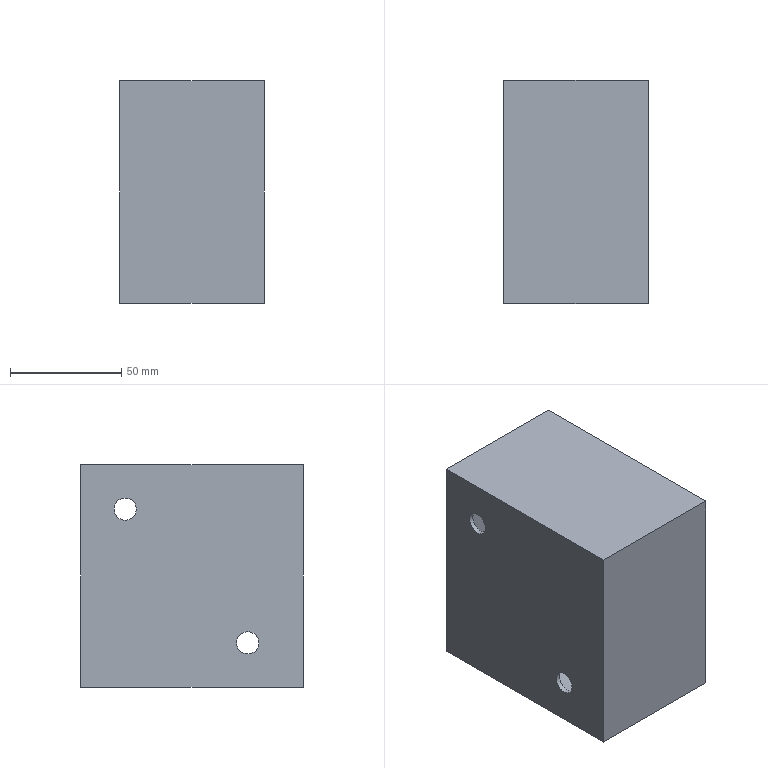Part | NX | features solid 2 | 1 solid | 18 faces | box 65 x 100 x 100 mm | volume 312986 mm3 | plane 16 | cylinder 2 | commonest cylinder face diameters 10 x2
STEP:
#1=CARTESIAN_POINT('',(1044.,-116.,-470.));
#2=VERTEX_POINT('',#1);
#3=CARTESIAN_POINT('',(1044.,-116.,-390.));
#4=VERTEX_POINT('',#3);
#5=CARTESIAN_POINT('',(1044.,-116.,-480.));
#6=DIRECTION('',(0.,0.,1.));
#7=VECTOR('',#6,1000.);
#8=LINE('',#5,#7);
#9=EDGE_CURVE('',#2,#4,#8,.T.);
#10=ORIENTED_EDGE('',*,*,#9,.T.);
#11=CARTESIAN_POINT('',(1044.,-196.,-390.));
#12=VERTEX_POINT('',#11);
#13=CARTESIAN_POINT('',(1044.,-206.,-390.));
#14=DIRECTION('',(0.,-1.,0.));
#15=VECTOR('',#14,1000.);
#16=LINE('',#13,#15);
#17=EDGE_CURVE('',#12,#4,#16,.F.);
#18=ORIENTED_EDGE('',*,*,#17,.F.);
#19=CARTESIAN_POINT('',(1044.,-196.,-470.));
#20=VERTEX_POINT('',#19);
#21=CARTESIAN_POINT('',(1044.,-196.,-480.));
#22=DIRECTION('',(0.,0.,-1.));
#23=VECTOR('',#22,1000.);
#24=LINE('',#21,#23);
#25=EDGE_CURVE('',#20,#12,#24,.F.);
#26=ORIENTED_EDGE('',*,*,#25,.F.);
#27=CARTESIAN_POINT('',(1044.,-206.,-470.));
#28=DIRECTION('',(0.,-1.,0.));
#29=VECTOR('',#28,1000.);
#30=LINE('',#27,#29);
#31=EDGE_CURVE('',#20,#2,#30,.F.);
#32=ORIENTED_EDGE('',*,*,#31,.T.);
#33=EDGE_LOOP('',(#10,#18,#26,#32));
#34=FACE_BOUND('',#33,.T.);
#35=CARTESIAN_POINT('',(1044.,-176.,-460.));
#36=VERTEX_POINT('',#35);
#37=CARTESIAN_POINT('',(1044.,-181.,-460.));
#38=DIRECTION('',(-1.,0.,0.));
#39=DIRECTION('',(0.,1.,0.));
#40=AXIS2_PLACEMENT_3D('',#37,#38,#39);
#41=CIRCLE('',#40,5.);
#42=EDGE_CURVE('',#36,#36,#41,.T.);
#43=ORIENTED_EDGE('',*,*,#42,.T.);
#44=EDGE_LOOP('',(#43));
#45=FACE_BOUND('',#44,.T.);
#46=CARTESIAN_POINT('',(1044.,-121.,-400.));
#47=VERTEX_POINT('',#46);
#48=CARTESIAN_POINT('',(1044.,-126.,-400.));
#49=DIRECTION('',(-1.,0.,0.));
#50=DIRECTION('',(0.,1.,0.));
#51=AXIS2_PLACEMENT_3D('',#48,#49,#50);
#52=CIRCLE('',#51,5.);
#53=EDGE_CURVE('',#47,#47,#52,.T.);
#54=ORIENTED_EDGE('',*,*,#53,.T.);
#55=EDGE_LOOP('',(#54));
#56=FACE_BOUND('',#55,.T.);
#57=CARTESIAN_POINT('',(1044.,-121.,-450.));
#58=VERTEX_POINT('',#57);
#59=CARTESIAN_POINT('',(1044.,-121.,-425.));
#60=VERTEX_POINT('',#59);
#61=CARTESIAN_POINT('',(1044.,-121.,-480.));
#62=DIRECTION('',(0.,0.,1.));
#63=VECTOR('',#62,1000.);
#64=LINE('',#61,#63);
#65=EDGE_CURVE('',#58,#60,#64,.T.);
#66=ORIENTED_EDGE('',*,*,#65,.F.);
#67=CARTESIAN_POINT('',(1044.,-191.,-450.));
#68=VERTEX_POINT('',#67);
#69=CARTESIAN_POINT('',(1044.,-106.,-450.));
#70=DIRECTION('',(0.,1.,0.));
#71=VECTOR('',#70,1000.);
#72=LINE('',#69,#71);
#73=EDGE_CURVE('',#68,#58,#72,.T.);
#74=ORIENTED_EDGE('',*,*,#73,.F.);
#75=CARTESIAN_POINT('',(1044.,-191.,-425.));
#76=VERTEX_POINT('',#75);
#77=CARTESIAN_POINT('',(1044.,-191.,-480.));
#78=DIRECTION('',(0.,0.,-1.));
#79=VECTOR('',#78,1000.);
#80=LINE('',#77,#79);
#81=EDGE_CURVE('',#76,#68,#80,.T.);
#82=ORIENTED_EDGE('',*,*,#81,.F.);
#83=CARTESIAN_POINT('',(1044.,-106.,-425.));
#84=DIRECTION('',(0.,-1.,0.));
#85=VECTOR('',#84,1000.);
#86=LINE('',#83,#85);
#87=EDGE_CURVE('',#60,#76,#86,.T.);
#88=ORIENTED_EDGE('',*,*,#87,.F.);
#89=EDGE_LOOP('',(#66,#74,#82,#88));
#90=FACE_BOUND('',#89,.T.);
#91=CARTESIAN_POINT('',(1044.,-106.,-480.));
#92=DIRECTION('',(-1.,0.,0.));
#93=DIRECTION('',(0.,1.,0.));
#94=AXIS2_PLACEMENT_3D('',#91,#92,#93);
#95=PLANE('',#94);
#96=ADVANCED_FACE('',(#34,#45,#56,#90),#95,.F.);
#97=ORIENTED_EDGE('',*,*,#25,.T.);
#98=CARTESIAN_POINT('',(1107.,-196.,-390.));
#99=VERTEX_POINT('',#98);
#100=CARTESIAN_POINT('',(1107.,-196.,-390.));
#101=DIRECTION('',(1.,0.,0.));
#102=VECTOR('',#101,1000.);
#103=LINE('',#100,#102);
#104=EDGE_CURVE('',#12,#99,#103,.T.);
#105=ORIENTED_EDGE('',*,*,#104,.T.);
#106=CARTESIAN_POINT('',(1107.,-196.,-470.));
#107=VERTEX_POINT('',#106);
#108=CARTESIAN_POINT('',(1107.,-196.,-480.));
#109=DIRECTION('',(0.,0.,1.));
#110=VECTOR('',#109,1000.);
#111=LINE('',#108,#110);
#112=EDGE_CURVE('',#107,#99,#111,.T.);
#113=ORIENTED_EDGE('',*,*,#112,.F.);
#114=CARTESIAN_POINT('',(1107.,-196.,-470.));
#115=DIRECTION('',(1.,0.,0.));
#116=VECTOR('',#115,1000.);
#117=LINE('',#114,#116);
#118=EDGE_CURVE('',#20,#107,#117,.T.);
#119=ORIENTED_EDGE('',*,*,#118,.F.);
#120=EDGE_LOOP('',(#97,#105,#113,#119));
#121=FACE_BOUND('',#120,.T.);
#122=CARTESIAN_POINT('',(1107.,-196.,-480.));
#123=DIRECTION('',(0.,-1.,0.));
#124=DIRECTION('',(-1.,0.,0.));
#125=AXIS2_PLACEMENT_3D('',#122,#123,#124);
#126=PLANE('',#125);
#127=ADVANCED_FACE('',(#121),#126,.F.);
#128=CARTESIAN_POINT('',(1107.,-206.,-480.));
#129=VERTEX_POINT('',#128);
#130=CARTESIAN_POINT('',(1107.,-106.,-480.));
#131=VERTEX_POINT('',#130);
#132=CARTESIAN_POINT('',(1107.,-206.,-480.));
#133=DIRECTION('',(0.,1.,0.));
#134=VECTOR('',#133,1000.);
#135=LINE('',#132,#134);
#136=EDGE_CURVE('',#129,#131,#135,.T.);
#137=ORIENTED_EDGE('',*,*,#136,.F.);
#138=CARTESIAN_POINT('',(1042.,-206.,-480.));
#139=VERTEX_POINT('',#138);
#140=CARTESIAN_POINT('',(1042.,-206.,-480.));
#141=DIRECTION('',(1.,0.,0.));
#142=VECTOR('',#141,1000.);
#143=LINE('',#140,#142);
#144=EDGE_CURVE('',#139,#129,#143,.T.);
#145=ORIENTED_EDGE('',*,*,#144,.F.);
#146=CARTESIAN_POINT('',(1042.,-106.,-480.));
#147=VERTEX_POINT('',#146);
#148=CARTESIAN_POINT('',(1042.,-106.,-480.));
#149=DIRECTION('',(0.,-1.,0.));
#150=VECTOR('',#149,1000.);
#151=LINE('',#148,#150);
#152=EDGE_CURVE('',#147,#139,#151,.T.);
#153=ORIENTED_EDGE('',*,*,#152,.F.);
#154=CARTESIAN_POINT('',(1042.,-106.,-480.));
#155=DIRECTION('',(1.,0.,0.));
#156=VECTOR('',#155,1000.);
#157=LINE('',#154,#156);
#158=EDGE_CURVE('',#147,#131,#157,.T.);
#159=ORIENTED_EDGE('',*,*,#158,.T.);
#160=EDGE_LOOP('',(#137,#145,#153,#159));
#161=FACE_BOUND('',#160,.T.);
#162=CARTESIAN_POINT('',(1042.,-106.,-480.));
#163=DIRECTION('',(0.,0.,-1.));
#164=DIRECTION('',(0.,-1.,0.));
#165=AXIS2_PLACEMENT_3D('',#162,#163,#164);
#166=PLANE('',#165);
#167=ADVANCED_FACE('',(#161),#166,.T.);
#168=ORIENTED_EDGE('',*,*,#158,.F.);
#169=CARTESIAN_POINT('',(1042.,-106.,-380.));
#170=VERTEX_POINT('',#169);
#171=CARTESIAN_POINT('',(1042.,-106.,-480.));
#172=DIRECTION('',(0.,0.,1.));
#173=VECTOR('',#172,1000.);
#174=LINE('',#171,#173);
#175=EDGE_CURVE('',#147,#170,#174,.T.);
#176=ORIENTED_EDGE('',*,*,#175,.T.);
#177=CARTESIAN_POINT('',(1107.,-106.,-380.));
#178=VERTEX_POINT('',#177);
#179=CARTESIAN_POINT('',(1042.,-106.,-380.));
#180=DIRECTION('',(1.,0.,0.));
#181=VECTOR('',#180,1000.);
#182=LINE('',#179,#181);
#183=EDGE_CURVE('',#170,#178,#182,.T.);
#184=ORIENTED_EDGE('',*,*,#183,.T.);
#185=CARTESIAN_POINT('',(1107.,-106.,-480.));
#186=DIRECTION('',(0.,0.,1.));
#187=VECTOR('',#186,1000.);
#188=LINE('',#185,#187);
#189=EDGE_CURVE('',#131,#178,#188,.T.);
#190=ORIENTED_EDGE('',*,*,#189,.F.);
#191=EDGE_LOOP('',(#168,#176,#184,#190));
#192=FACE_BOUND('',#191,.T.);
#193=CARTESIAN_POINT('',(1042.,-106.,-480.));
#194=DIRECTION('',(0.,-1.,0.));
#195=DIRECTION('',(0.,0.,1.));
#196=AXIS2_PLACEMENT_3D('',#193,#194,#195);
#197=PLANE('',#196);
#198=ADVANCED_FACE('',(#192),#197,.F.);
#199=CARTESIAN_POINT('',(1107.,-206.,-380.));
#200=VERTEX_POINT('',#199);
#201=CARTESIAN_POINT('',(1107.,-206.,-380.));
#202=DIRECTION('',(0.,1.,0.));
#203=VECTOR('',#202,1000.);
#204=LINE('',#201,#203);
#205=EDGE_CURVE('',#200,#178,#204,.T.);
#206=ORIENTED_EDGE('',*,*,#205,.T.);
#207=ORIENTED_EDGE('',*,*,#183,.F.);
#208=CARTESIAN_POINT('',(1042.,-206.,-380.));
#209=VERTEX_POINT('',#208);
#210=CARTESIAN_POINT('',(1042.,-106.,-380.));
#211=DIRECTION('',(0.,-1.,0.));
#212=VECTOR('',#211,1000.);
#213=LINE('',#210,#212);
#214=EDGE_CURVE('',#170,#209,#213,.T.);
#215=ORIENTED_EDGE('',*,*,#214,.T.);
#216=CARTESIAN_POINT('',(1042.,-206.,-380.));
#217=DIRECTION('',(1.,0.,0.));
#218=VECTOR('',#217,1000.);
#219=LINE('',#216,#218);
#220=EDGE_CURVE('',#209,#200,#219,.T.);
#221=ORIENTED_EDGE('',*,*,#220,.T.);
#222=EDGE_LOOP('',(#206,#207,#215,#221));
#223=FACE_BOUND('',#222,.T.);
#224=CARTESIAN_POINT('',(1042.,-106.,-380.));
#225=DIRECTION('',(0.,0.,-1.));
#226=DIRECTION('',(0.,-1.,0.));
#227=AXIS2_PLACEMENT_3D('',#224,#225,#226);
#228=PLANE('',#227);
#229=ADVANCED_FACE('',(#223),#228,.F.);
#230=CARTESIAN_POINT('',(1107.,-206.,-480.));
#231=DIRECTION('',(0.,0.,1.));
#232=VECTOR('',#231,1000.);
#233=LINE('',#230,#232);
#234=EDGE_CURVE('',#129,#200,#233,.T.);
#235=ORIENTED_EDGE('',*,*,#234,.T.);
#236=ORIENTED_EDGE('',*,*,#220,.F.);
#237=CARTESIAN_POINT('',(1042.,-206.,-480.));
#238=DIRECTION('',(0.,0.,1.));
#239=VECTOR('',#238,1000.);
#240=LINE('',#237,#239);
#241=EDGE_CURVE('',#139,#209,#240,.T.);
#242=ORIENTED_EDGE('',*,*,#241,.F.);
#243=ORIENTED_EDGE('',*,*,#144,.T.);
#244=EDGE_LOOP('',(#235,#236,#242,#243));
#245=FACE_BOUND('',#244,.T.);
#246=CARTESIAN_POINT('',(1042.,-206.,-480.));
#247=DIRECTION('',(0.,-1.,0.));
#248=DIRECTION('',(0.,0.,1.));
#249=AXIS2_PLACEMENT_3D('',#246,#247,#248);
#250=PLANE('',#249);
#251=ADVANCED_FACE('',(#245),#250,.T.);
#252=ORIENTED_EDGE('',*,*,#214,.F.);
#253=ORIENTED_EDGE('',*,*,#175,.F.);
#254=ORIENTED_EDGE('',*,*,#152,.T.);
#255=ORIENTED_EDGE('',*,*,#241,.T.);
#256=EDGE_LOOP('',(#252,#253,#254,#255));
#257=FACE_BOUND('',#256,.T.);
#258=CARTESIAN_POINT('',(1042.,-176.,-460.));
#259=VERTEX_POINT('',#258);
#260=CARTESIAN_POINT('',(1042.,-181.,-460.));
#261=DIRECTION('',(-1.,0.,0.));
#262=DIRECTION('',(0.,1.,0.));
#263=AXIS2_PLACEMENT_3D('',#260,#261,#262);
#264=CIRCLE('',#263,5.);
#265=EDGE_CURVE('',#259,#259,#264,.T.);
#266=ORIENTED_EDGE('',*,*,#265,.F.);
#267=EDGE_LOOP('',(#266));
#268=FACE_BOUND('',#267,.T.);
#269=CARTESIAN_POINT('',(1042.,-121.,-400.));
#270=VERTEX_POINT('',#269);
#271=CARTESIAN_POINT('',(1042.,-126.,-400.));
#272=DIRECTION('',(-1.,0.,0.));
#273=DIRECTION('',(0.,1.,0.));
#274=AXIS2_PLACEMENT_3D('',#271,#272,#273);
#275=CIRCLE('',#274,5.);
#276=EDGE_CURVE('',#270,#270,#275,.T.);
#277=ORIENTED_EDGE('',*,*,#276,.F.);
#278=EDGE_LOOP('',(#277));
#279=FACE_BOUND('',#278,.T.);
#280=CARTESIAN_POINT('',(1042.,-106.,-480.));
#281=DIRECTION('',(-1.,0.,0.));
#282=DIRECTION('',(0.,1.,0.));
#283=AXIS2_PLACEMENT_3D('',#280,#281,#282);
#284=PLANE('',#283);
#285=ADVANCED_FACE('',(#257,#268,#279),#284,.T.);
#286=ORIENTED_EDGE('',*,*,#112,.T.);
#287=CARTESIAN_POINT('',(1107.,-116.,-390.));
#288=VERTEX_POINT('',#287);
#289=CARTESIAN_POINT('',(1107.,-206.,-390.));
#290=DIRECTION('',(0.,-1.,0.));
#291=VECTOR('',#290,1000.);
#292=LINE('',#289,#291);
#293=EDGE_CURVE('',#99,#288,#292,.F.);
#294=ORIENTED_EDGE('',*,*,#293,.T.);
#295=CARTESIAN_POINT('',(1107.,-116.,-470.));
#296=VERTEX_POINT('',#295);
#297=CARTESIAN_POINT('',(1107.,-116.,-480.));
#298=DIRECTION('',(0.,0.,-1.));
#299=VECTOR('',#298,1000.);
#300=LINE('',#297,#299);
#301=EDGE_CURVE('',#296,#288,#300,.F.);
#302=ORIENTED_EDGE('',*,*,#301,.F.);
#303=CARTESIAN_POINT('',(1107.,-206.,-470.));
#304=DIRECTION('',(0.,-1.,0.));
#305=VECTOR('',#304,1000.);
#306=LINE('',#303,#305);
#307=EDGE_CURVE('',#107,#296,#306,.F.);
#308=ORIENTED_EDGE('',*,*,#307,.F.);
#309=EDGE_LOOP('',(#286,#294,#302,#308));
#310=FACE_BOUND('',#309,.T.);
#311=ORIENTED_EDGE('',*,*,#189,.T.);
#312=ORIENTED_EDGE('',*,*,#205,.F.);
#313=ORIENTED_EDGE('',*,*,#234,.F.);
#314=ORIENTED_EDGE('',*,*,#136,.T.);
#315=EDGE_LOOP('',(#311,#312,#313,#314));
#316=FACE_BOUND('',#315,.T.);
#317=CARTESIAN_POINT('',(1107.,-206.,-480.));
#318=DIRECTION('',(1.,0.,0.));
#319=DIRECTION('',(0.,0.,1.));
#320=AXIS2_PLACEMENT_3D('',#317,#318,#319);
#321=PLANE('',#320);
#322=ADVANCED_FACE('',(#310,#316),#321,.T.);
#323=ORIENTED_EDGE('',*,*,#31,.F.);
#324=ORIENTED_EDGE('',*,*,#118,.T.);
#325=ORIENTED_EDGE('',*,*,#307,.T.);
#326=CARTESIAN_POINT('',(1107.,-116.,-470.));
#327=DIRECTION('',(1.,0.,0.));
#328=VECTOR('',#327,1000.);
#329=LINE('',#326,#328);
#330=EDGE_CURVE('',#296,#2,#329,.F.);
#331=ORIENTED_EDGE('',*,*,#330,.T.);
#332=EDGE_LOOP('',(#323,#324,#325,#331));
#333=FACE_BOUND('',#332,.T.);
#334=CARTESIAN_POINT('',(1107.,-206.,-470.));
#335=DIRECTION('',(0.,0.,-1.));
#336=DIRECTION('',(1.,0.,0.));
#337=AXIS2_PLACEMENT_3D('',#334,#335,#336);
#338=PLANE('',#337);
#339=ADVANCED_FACE('',(#333),#338,.F.);
#340=CARTESIAN_POINT('',(1107.,-116.,-390.));
#341=DIRECTION('',(1.,0.,0.));
#342=VECTOR('',#341,1000.);
#343=LINE('',#340,#342);
#344=EDGE_CURVE('',#288,#4,#343,.F.);
#345=ORIENTED_EDGE('',*,*,#344,.T.);
#346=ORIENTED_EDGE('',*,*,#9,.F.);
#347=ORIENTED_EDGE('',*,*,#330,.F.);
#348=ORIENTED_EDGE('',*,*,#301,.T.);
#349=EDGE_LOOP('',(#345,#346,#347,#348));
#350=FACE_BOUND('',#349,.T.);
#351=CARTESIAN_POINT('',(1107.,-116.,-480.));
#352=DIRECTION('',(0.,-1.,0.));
#353=DIRECTION('',(-1.,0.,0.));
#354=AXIS2_PLACEMENT_3D('',#351,#352,#353);
#355=PLANE('',#354);
#356=ADVANCED_FACE('',(#350),#355,.T.);
#357=ORIENTED_EDGE('',*,*,#104,.F.);
#358=ORIENTED_EDGE('',*,*,#17,.T.);
#359=ORIENTED_EDGE('',*,*,#344,.F.);
#360=ORIENTED_EDGE('',*,*,#293,.F.);
#361=EDGE_LOOP('',(#357,#358,#359,#360));
#362=FACE_BOUND('',#361,.T.);
#363=CARTESIAN_POINT('',(1107.,-206.,-390.));
#364=DIRECTION('',(0.,0.,-1.));
#365=DIRECTION('',(1.,0.,0.));
#366=AXIS2_PLACEMENT_3D('',#363,#364,#365);
#367=PLANE('',#366);
#368=ADVANCED_FACE('',(#362),#367,.T.);
#369=ORIENTED_EDGE('',*,*,#265,.T.);
#370=EDGE_LOOP('',(#369));
#371=FACE_BOUND('',#370,.T.);
#372=ORIENTED_EDGE('',*,*,#42,.F.);
#373=EDGE_LOOP('',(#372));
#374=FACE_BOUND('',#373,.T.);
#375=CARTESIAN_POINT('',(1044.,-181.,-460.));
#376=DIRECTION('',(-1.,0.,0.));
#377=DIRECTION('',(0.,1.,0.));
#378=AXIS2_PLACEMENT_3D('',#375,#376,#377);
#379=CYLINDRICAL_SURFACE('',#378,5.);
#380=ADVANCED_FACE('',(#371,#374),#379,.F.);
#381=ORIENTED_EDGE('',*,*,#276,.T.);
#382=EDGE_LOOP('',(#381));
#383=FACE_BOUND('',#382,.T.);
#384=ORIENTED_EDGE('',*,*,#53,.F.);
#385=EDGE_LOOP('',(#384));
#386=FACE_BOUND('',#385,.T.);
#387=CARTESIAN_POINT('',(1044.,-126.,-400.));
#388=DIRECTION('',(-1.,0.,0.));
#389=DIRECTION('',(0.,1.,0.));
#390=AXIS2_PLACEMENT_3D('',#387,#388,#389);
#391=CYLINDRICAL_SURFACE('',#390,5.);
#392=ADVANCED_FACE('',(#383,#386),#391,.F.);
#393=CARTESIAN_POINT('',(1082.,-121.,-450.));
#394=VERTEX_POINT('',#393);
#395=CARTESIAN_POINT('',(1052.,-121.,-450.));
#396=DIRECTION('',(1.,0.,0.));
#397=VECTOR('',#396,1000.);
#398=LINE('',#395,#397);
#399=EDGE_CURVE('',#58,#394,#398,.T.);
#400=ORIENTED_EDGE('',*,*,#399,.F.);
#401=ORIENTED_EDGE('',*,*,#65,.T.);
#402=CARTESIAN_POINT('',(1082.,-121.,-425.));
#403=VERTEX_POINT('',#402);
#404=CARTESIAN_POINT('',(1052.,-121.,-425.));
#405=DIRECTION('',(1.,0.,0.));
#406=VECTOR('',#405,1000.);
#407=LINE('',#404,#406);
#408=EDGE_CURVE('',#60,#403,#407,.T.);
#409=ORIENTED_EDGE('',*,*,#408,.T.);
#410=CARTESIAN_POINT('',(1082.,-121.,-435.));
#411=DIRECTION('',(0.,0.,-1.));
#412=VECTOR('',#411,1000.);
#413=LINE('',#410,#412);
#414=EDGE_CURVE('',#403,#394,#413,.T.);
#415=ORIENTED_EDGE('',*,*,#414,.T.);
#416=EDGE_LOOP('',(#400,#401,#409,#415));
#417=FACE_BOUND('',#416,.T.);
#418=CARTESIAN_POINT('',(1052.,-121.,-435.));
#419=DIRECTION('',(0.,-1.,0.));
#420=DIRECTION('',(-1.,0.,0.));
#421=AXIS2_PLACEMENT_3D('',#418,#419,#420);
#422=PLANE('',#421);
#423=ADVANCED_FACE('',(#417),#422,.F.);
#424=CARTESIAN_POINT('',(1082.,-191.,-450.));
#425=VERTEX_POINT('',#424);
#426=CARTESIAN_POINT('',(1052.,-191.,-450.));
#427=DIRECTION('',(1.,0.,0.));
#428=VECTOR('',#427,1000.);
#429=LINE('',#426,#428);
#430=EDGE_CURVE('',#68,#425,#429,.T.);
#431=ORIENTED_EDGE('',*,*,#430,.F.);
#432=ORIENTED_EDGE('',*,*,#73,.T.);
#433=ORIENTED_EDGE('',*,*,#399,.T.);
#434=CARTESIAN_POINT('',(1082.,-121.,-450.));
#435=DIRECTION('',(0.,-1.,0.));
#436=VECTOR('',#435,1000.);
#437=LINE('',#434,#436);
#438=EDGE_CURVE('',#394,#425,#437,.T.);
#439=ORIENTED_EDGE('',*,*,#438,.T.);
#440=EDGE_LOOP('',(#431,#432,#433,#439));
#441=FACE_BOUND('',#440,.T.);
#442=CARTESIAN_POINT('',(1052.,-121.,-450.));
#443=DIRECTION('',(0.,0.,1.));
#444=DIRECTION('',(-1.,0.,0.));
#445=AXIS2_PLACEMENT_3D('',#442,#443,#444);
#446=PLANE('',#445);
#447=ADVANCED_FACE('',(#441),#446,.F.);
#448=CARTESIAN_POINT('',(1082.,-191.,-425.));
#449=VERTEX_POINT('',#448);
#450=CARTESIAN_POINT('',(1052.,-191.,-425.));
#451=DIRECTION('',(1.,0.,0.));
#452=VECTOR('',#451,1000.);
#453=LINE('',#450,#452);
#454=EDGE_CURVE('',#76,#449,#453,.T.);
#455=ORIENTED_EDGE('',*,*,#454,.F.);
#456=ORIENTED_EDGE('',*,*,#81,.T.);
#457=ORIENTED_EDGE('',*,*,#430,.T.);
#458=CARTESIAN_POINT('',(1082.,-191.,-460.));
#459=DIRECTION('',(0.,0.,1.));
#460=VECTOR('',#459,1000.);
#461=LINE('',#458,#460);
#462=EDGE_CURVE('',#425,#449,#461,.T.);
#463=ORIENTED_EDGE('',*,*,#462,.T.);
#464=EDGE_LOOP('',(#455,#456,#457,#463));
#465=FACE_BOUND('',#464,.T.);
#466=CARTESIAN_POINT('',(1052.,-191.,-460.));
#467=DIRECTION('',(0.,1.,0.));
#468=DIRECTION('',(1.,0.,0.));
#469=AXIS2_PLACEMENT_3D('',#466,#467,#468);
#470=PLANE('',#469);
#471=ADVANCED_FACE('',(#465),#470,.F.);
#472=ORIENTED_EDGE('',*,*,#408,.F.);
#473=ORIENTED_EDGE('',*,*,#87,.T.);
#474=ORIENTED_EDGE('',*,*,#454,.T.);
#475=CARTESIAN_POINT('',(1082.,-191.,-425.));
#476=DIRECTION('',(0.,1.,0.));
#477=VECTOR('',#476,1000.);
#478=LINE('',#475,#477);
#479=EDGE_CURVE('',#449,#403,#478,.T.);
#480=ORIENTED_EDGE('',*,*,#479,.T.);
#481=EDGE_LOOP('',(#472,#473,#474,#480));
#482=FACE_BOUND('',#481,.T.);
#483=CARTESIAN_POINT('',(1052.,-191.,-425.));
#484=DIRECTION('',(0.,0.,-1.));
#485=DIRECTION('',(1.,0.,0.));
#486=AXIS2_PLACEMENT_3D('',#483,#484,#485);
#487=PLANE('',#486);
#488=ADVANCED_FACE('',(#482),#487,.F.);
#489=ORIENTED_EDGE('',*,*,#414,.F.);
#490=ORIENTED_EDGE('',*,*,#479,.F.);
#491=ORIENTED_EDGE('',*,*,#462,.F.);
#492=ORIENTED_EDGE('',*,*,#438,.F.);
#493=EDGE_LOOP('',(#489,#490,#491,#492));
#494=FACE_BOUND('',#493,.T.);
#495=CARTESIAN_POINT('',(1082.,-121.,-460.));
#496=DIRECTION('',(-1.,0.,0.));
#497=DIRECTION('',(0.,1.,0.));
#498=AXIS2_PLACEMENT_3D('',#495,#496,#497);
#499=PLANE('',#498);
#500=ADVANCED_FACE('',(#494),#499,.F.);
#501=CLOSED_SHELL('',(#96,#127,#167,#198,#229,#251,#285,#322,#339,#356,#368,#380,#392,#423,#447,#471,#488,#500));
#502=MANIFOLD_SOLID_BREP('',#501);
#503=(LENGTH_UNIT()NAMED_UNIT(*)SI_UNIT(.MILLI.,.METRE.));
#504=UNCERTAINTY_MEASURE_WITH_UNIT(LENGTH_MEASURE(0.00001),#503,'','');
#505=(NAMED_UNIT(*)PLANE_ANGLE_UNIT()SI_UNIT($,.RADIAN.));
#506=(NAMED_UNIT(*)SI_UNIT($,.STERADIAN.)SOLID_ANGLE_UNIT());
#507=(GEOMETRIC_REPRESENTATION_CONTEXT(3)GLOBAL_UNCERTAINTY_ASSIGNED_CONTEXT((#504))GLOBAL_UNIT_ASSIGNED_CONTEXT((#503,#505,#506))REPRESENTATION_CONTEXT('',''));
#508=ADVANCED_BREP_SHAPE_REPRESENTATION('',(#502),#507);